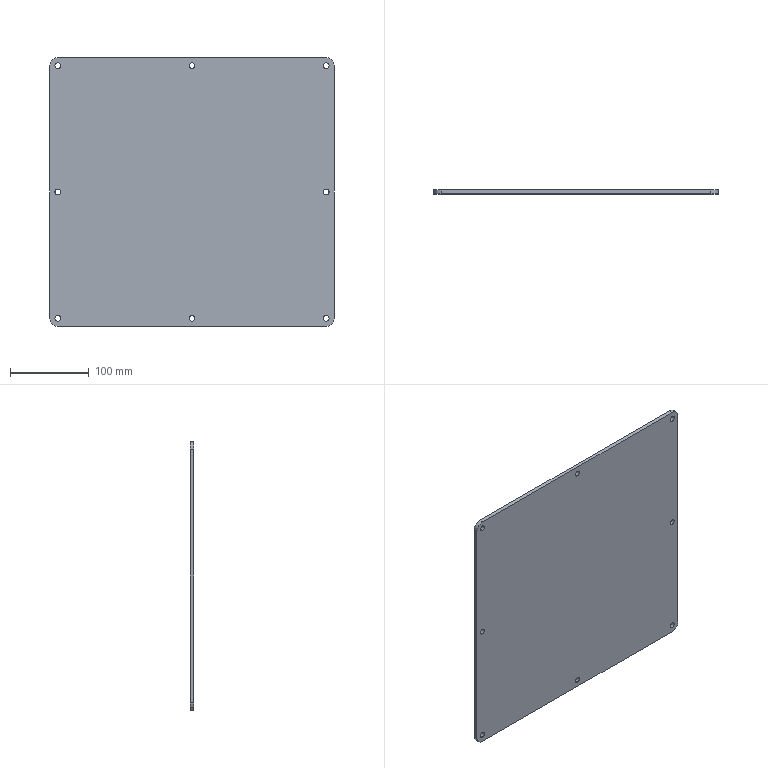Part | STEP file | b-007 | 1 solid | 26 faces | box 360 x 5 x 340 mm | volume 610031 mm3 | cylinder 20 | plane 6 | commonest cylinder face diameters 7 x16 20 x4